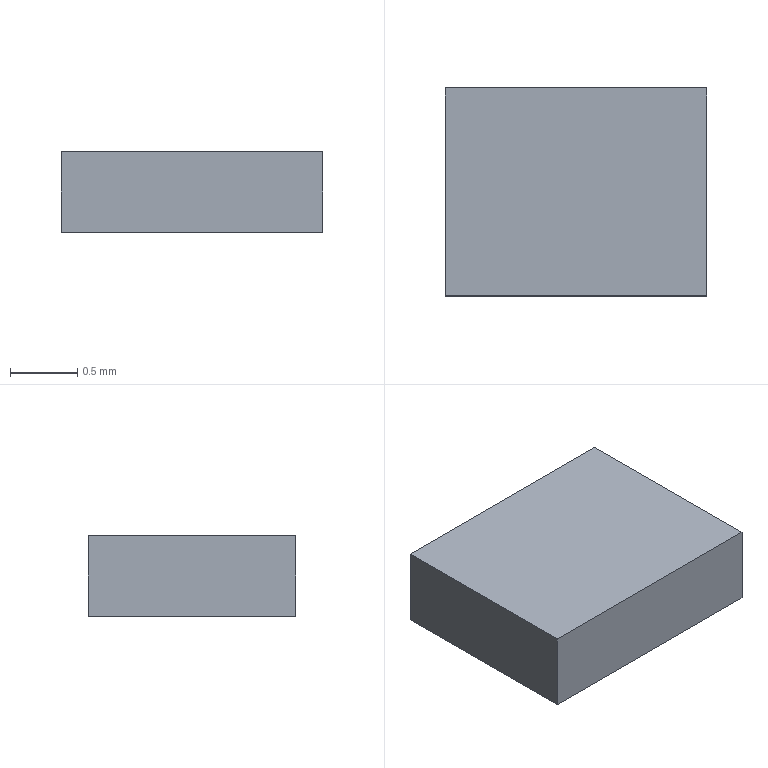Part | Creo | 1 solid | 6 faces | box 1.95 x 1.55 x 0.6 mm | volume 1.813 mm3 | plane 6
STEP:
#1=CARTESIAN_POINT('',(0.,0.,0.));
#2=DIRECTION('',(0.,0.,1.));
#3=DIRECTION('',(1.,0.,0.));
#4=AXIS2_PLACEMENT_3D('',#1,#2,#3);
#5=CARTESIAN_POINT('',(-1.025,-0.825,0.));
#6=VERTEX_POINT('',#5);
#7=CARTESIAN_POINT('',(0.925,-0.825,0.));
#8=VERTEX_POINT('',#7);
#9=CARTESIAN_POINT('',(-1.025,-0.825,0.));
#10=DIRECTION('',(1.,0.,0.));
#11=VECTOR('',#10,1.95);
#12=LINE('',#9,#11);
#13=EDGE_CURVE('',#6,#8,#12,.T.);
#14=ORIENTED_EDGE('',*,*,#13,.T.);
#15=CARTESIAN_POINT('',(0.925,0.725,0.));
#16=VERTEX_POINT('',#15);
#17=CARTESIAN_POINT('',(0.925,-0.825,0.));
#18=DIRECTION('',(0.,1.,0.));
#19=VECTOR('',#18,1.55);
#20=LINE('',#17,#19);
#21=EDGE_CURVE('',#8,#16,#20,.T.);
#22=ORIENTED_EDGE('',*,*,#21,.T.);
#23=CARTESIAN_POINT('',(-1.025,0.725,0.));
#24=VERTEX_POINT('',#23);
#25=CARTESIAN_POINT('',(0.925,0.725,0.));
#26=DIRECTION('',(-1.,0.,0.));
#27=VECTOR('',#26,1.95);
#28=LINE('',#25,#27);
#29=EDGE_CURVE('',#16,#24,#28,.T.);
#30=ORIENTED_EDGE('',*,*,#29,.T.);
#31=CARTESIAN_POINT('',(-1.025,0.725,0.));
#32=DIRECTION('',(0.,-1.,0.));
#33=VECTOR('',#32,1.55);
#34=LINE('',#31,#33);
#35=EDGE_CURVE('',#24,#6,#34,.T.);
#36=ORIENTED_EDGE('',*,*,#35,.T.);
#37=EDGE_LOOP('',(#14,#22,#30,#36));
#38=FACE_OUTER_BOUND('',#37,.F.);
#39=CARTESIAN_POINT('',(0.,0.,0.));
#40=DIRECTION('',(0.,0.,1.));
#41=DIRECTION('',(1.,0.,0.));
#42=AXIS2_PLACEMENT_3D('',#39,#40,#41);
#43=PLANE('',#42);
#44=ADVANCED_FACE('',(#38),#43,.F.);
#45=ORIENTED_EDGE('',*,*,#13,.F.);
#46=CARTESIAN_POINT('',(-1.025,-0.825,0.6));
#47=VERTEX_POINT('',#46);
#48=CARTESIAN_POINT('',(-1.025,-0.825,0.));
#49=DIRECTION('',(0.,0.,1.));
#50=VECTOR('',#49,0.6);
#51=LINE('',#48,#50);
#52=EDGE_CURVE('',#6,#47,#51,.T.);
#53=ORIENTED_EDGE('',*,*,#52,.T.);
#54=CARTESIAN_POINT('',(0.925,-0.825,0.6));
#55=VERTEX_POINT('',#54);
#56=CARTESIAN_POINT('',(-1.025,-0.825,0.6));
#57=DIRECTION('',(1.,0.,0.));
#58=VECTOR('',#57,1.95);
#59=LINE('',#56,#58);
#60=EDGE_CURVE('',#47,#55,#59,.T.);
#61=ORIENTED_EDGE('',*,*,#60,.T.);
#62=CARTESIAN_POINT('',(0.925,-0.825,0.));
#63=DIRECTION('',(0.,0.,1.));
#64=VECTOR('',#63,0.6);
#65=LINE('',#62,#64);
#66=EDGE_CURVE('',#8,#55,#65,.T.);
#67=ORIENTED_EDGE('',*,*,#66,.F.);
#68=EDGE_LOOP('',(#45,#53,#61,#67));
#69=FACE_OUTER_BOUND('',#68,.F.);
#70=CARTESIAN_POINT('',(-1.025,-0.825,0.));
#71=DIRECTION('',(0.,-1.,0.));
#72=DIRECTION('',(1.,0.,0.));
#73=AXIS2_PLACEMENT_3D('',#70,#71,#72);
#74=PLANE('',#73);
#75=ADVANCED_FACE('',(#69),#74,.T.);
#76=ORIENTED_EDGE('',*,*,#35,.F.);
#77=CARTESIAN_POINT('',(-1.025,0.725,0.6));
#78=VERTEX_POINT('',#77);
#79=CARTESIAN_POINT('',(-1.025,0.725,0.));
#80=DIRECTION('',(0.,0.,1.));
#81=VECTOR('',#80,0.6);
#82=LINE('',#79,#81);
#83=EDGE_CURVE('',#24,#78,#82,.T.);
#84=ORIENTED_EDGE('',*,*,#83,.T.);
#85=CARTESIAN_POINT('',(-1.025,0.725,0.6));
#86=DIRECTION('',(0.,-1.,0.));
#87=VECTOR('',#86,1.55);
#88=LINE('',#85,#87);
#89=EDGE_CURVE('',#78,#47,#88,.T.);
#90=ORIENTED_EDGE('',*,*,#89,.T.);
#91=ORIENTED_EDGE('',*,*,#52,.F.);
#92=EDGE_LOOP('',(#76,#84,#90,#91));
#93=FACE_OUTER_BOUND('',#92,.F.);
#94=CARTESIAN_POINT('',(-1.025,0.725,0.));
#95=DIRECTION('',(-1.,0.,0.));
#96=DIRECTION('',(0.,-1.,0.));
#97=AXIS2_PLACEMENT_3D('',#94,#95,#96);
#98=PLANE('',#97);
#99=ADVANCED_FACE('',(#93),#98,.T.);
#100=ORIENTED_EDGE('',*,*,#29,.F.);
#101=CARTESIAN_POINT('',(0.925,0.725,0.6));
#102=VERTEX_POINT('',#101);
#103=CARTESIAN_POINT('',(0.925,0.725,0.));
#104=DIRECTION('',(0.,0.,1.));
#105=VECTOR('',#104,0.6);
#106=LINE('',#103,#105);
#107=EDGE_CURVE('',#16,#102,#106,.T.);
#108=ORIENTED_EDGE('',*,*,#107,.T.);
#109=CARTESIAN_POINT('',(0.925,0.725,0.6));
#110=DIRECTION('',(-1.,0.,0.));
#111=VECTOR('',#110,1.95);
#112=LINE('',#109,#111);
#113=EDGE_CURVE('',#102,#78,#112,.T.);
#114=ORIENTED_EDGE('',*,*,#113,.T.);
#115=ORIENTED_EDGE('',*,*,#83,.F.);
#116=EDGE_LOOP('',(#100,#108,#114,#115));
#117=FACE_OUTER_BOUND('',#116,.F.);
#118=CARTESIAN_POINT('',(0.925,0.725,0.));
#119=DIRECTION('',(0.,1.,0.));
#120=DIRECTION('',(-1.,0.,0.));
#121=AXIS2_PLACEMENT_3D('',#118,#119,#120);
#122=PLANE('',#121);
#123=ADVANCED_FACE('',(#117),#122,.T.);
#124=ORIENTED_EDGE('',*,*,#21,.F.);
#125=ORIENTED_EDGE('',*,*,#66,.T.);
#126=CARTESIAN_POINT('',(0.925,-0.825,0.6));
#127=DIRECTION('',(0.,1.,0.));
#128=VECTOR('',#127,1.55);
#129=LINE('',#126,#128);
#130=EDGE_CURVE('',#55,#102,#129,.T.);
#131=ORIENTED_EDGE('',*,*,#130,.T.);
#132=ORIENTED_EDGE('',*,*,#107,.F.);
#133=EDGE_LOOP('',(#124,#125,#131,#132));
#134=FACE_OUTER_BOUND('',#133,.F.);
#135=CARTESIAN_POINT('',(0.925,-0.825,0.));
#136=DIRECTION('',(1.,0.,0.));
#137=DIRECTION('',(0.,1.,0.));
#138=AXIS2_PLACEMENT_3D('',#135,#136,#137);
#139=PLANE('',#138);
#140=ADVANCED_FACE('',(#134),#139,.T.);
#141=ORIENTED_EDGE('',*,*,#60,.F.);
#142=ORIENTED_EDGE('',*,*,#89,.F.);
#143=ORIENTED_EDGE('',*,*,#113,.F.);
#144=ORIENTED_EDGE('',*,*,#130,.F.);
#145=EDGE_LOOP('',(#141,#142,#143,#144));
#146=FACE_OUTER_BOUND('',#145,.F.);
#147=CARTESIAN_POINT('',(0.,0.,0.6));
#148=DIRECTION('',(0.,0.,1.));
#149=DIRECTION('',(1.,0.,0.));
#150=AXIS2_PLACEMENT_3D('',#147,#148,#149);
#151=PLANE('',#150);
#152=ADVANCED_FACE('',(#146),#151,.T.);
#153=CLOSED_SHELL('',(#44,#75,#99,#123,#140,#152));
#154=MANIFOLD_SOLID_BREP('',#153);
#155=(LENGTH_UNIT()NAMED_UNIT(*)SI_UNIT(.MILLI.,.METRE.));
#156=UNCERTAINTY_MEASURE_WITH_UNIT(LENGTH_MEASURE(0.0002562),#155,'','');
#157=(NAMED_UNIT(*)PLANE_ANGLE_UNIT()SI_UNIT($,.RADIAN.));
#158=PLANE_ANGLE_MEASURE_WITH_UNIT(PLANE_ANGLE_MEASURE(0.01745),#157);
#159=(CONVERSION_BASED_UNIT('DEGREE',#158)NAMED_UNIT(*)PLANE_ANGLE_UNIT());
#160=(NAMED_UNIT(*)SI_UNIT($,.STERADIAN.)SOLID_ANGLE_UNIT());
#161=(GEOMETRIC_REPRESENTATION_CONTEXT(3)GLOBAL_UNCERTAINTY_ASSIGNED_CONTEXT((#156))GLOBAL_UNIT_ASSIGNED_CONTEXT((#155,#159,#160))REPRESENTATION_CONTEXT('',''));
#162=ADVANCED_BREP_SHAPE_REPRESENTATION('',(#4,#154),#161);